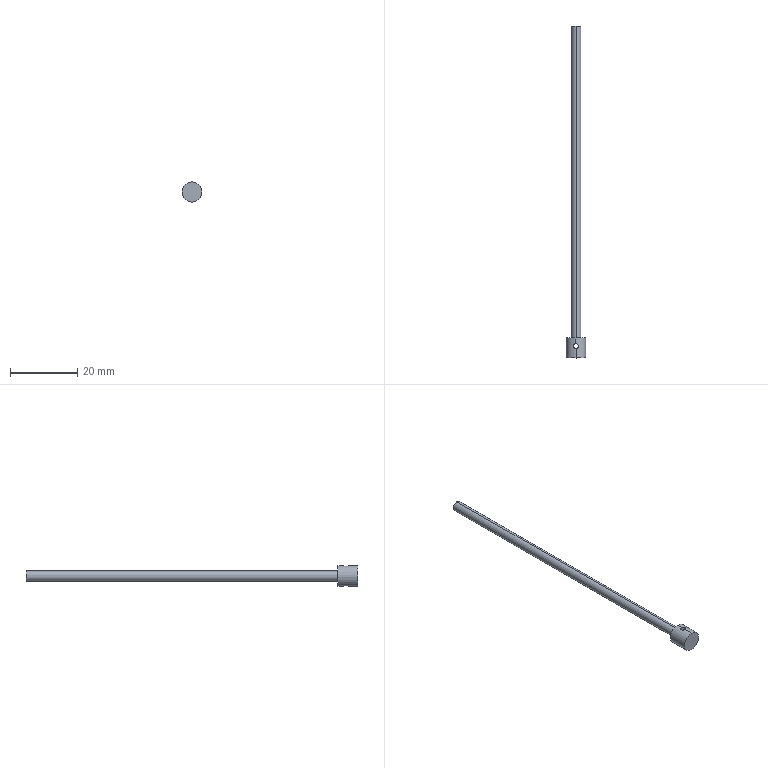Part | STEP file | magnetic tile detection pin | 1 solid | 9 faces | box 6 x 99 x 6 mm | volume 816.507 mm3 | cylinder 6 | plane 3 | commonest cylinder face diameters 1.5 x2 3 x2 6 x2
STEP:
#1=CARTESIAN_POINT('',(0.,0.,0.));
#2=DIRECTION('',(0.,0.,1.));
#3=DIRECTION('',(1.,0.,0.));
#4=AXIS2_PLACEMENT_3D('',#1,#2,#3);
#5=CARTESIAN_POINT('',(0.75,3.5,-2.905));
#6=VERTEX_POINT('',#5);
#7=CARTESIAN_POINT('',(0.,2.75,-3.));
#8=VERTEX_POINT('',#7);
#9=CARTESIAN_POINT('',(0.75,3.5,-2.905));
#10=CARTESIAN_POINT('',(0.75,3.402,-2.905));
#11=CARTESIAN_POINT('',(0.7304,3.303,-2.91));
#12=CARTESIAN_POINT('',(0.6548,3.121,-2.928));
#13=CARTESIAN_POINT('',(0.5996,3.039,-2.94));
#14=CARTESIAN_POINT('',(0.4606,2.9,-2.965));
#15=CARTESIAN_POINT('',(0.378,2.845,-2.977));
#16=CARTESIAN_POINT('',(0.1969,2.77,-2.995));
#17=CARTESIAN_POINT('',(0.0981,2.75,-3.));
#18=CARTESIAN_POINT('',(0.,2.75,-3.));
#19=B_SPLINE_CURVE_WITH_KNOTS('',3,(#9,#10,#11,#12,#13,#14,#15,#16,#17,#18),.UNSPECIFIED.,.F.,.F.,(4,2,2,2,4),(0.001177,0.001472,0.001766,0.00206,0.002354),.UNSPECIFIED.);
#20=CARTESIAN_POINT('',(0.,3.5,-5.));
#21=DIRECTION('',(0.,0.,1.));
#22=DIRECTION('',(1.,0.,0.));
#23=AXIS2_PLACEMENT_3D('',#20,#21,#22);
#24=CYLINDRICAL_SURFACE('',#23,0.75);
#25=CARTESIAN_POINT('',(6.283,2.095));
#26=CARTESIAN_POINT('',(6.259,2.095));
#27=CARTESIAN_POINT('',(6.212,2.095));
#28=CARTESIAN_POINT('',(6.14,2.093));
#29=CARTESIAN_POINT('',(6.069,2.091));
#30=CARTESIAN_POINT('',(5.997,2.088));
#31=CARTESIAN_POINT('',(5.925,2.084));
#32=CARTESIAN_POINT('',(5.854,2.079));
#33=CARTESIAN_POINT('',(5.782,2.073));
#34=CARTESIAN_POINT('',(5.711,2.067));
#35=CARTESIAN_POINT('',(5.64,2.061));
#36=CARTESIAN_POINT('',(5.569,2.054));
#37=CARTESIAN_POINT('',(5.497,2.047));
#38=CARTESIAN_POINT('',(5.426,2.04));
#39=CARTESIAN_POINT('',(5.355,2.034));
#40=CARTESIAN_POINT('',(5.284,2.027));
#41=CARTESIAN_POINT('',(5.213,2.022));
#42=CARTESIAN_POINT('',(5.141,2.016));
#43=CARTESIAN_POINT('',(5.07,2.011));
#44=CARTESIAN_POINT('',(4.999,2.007));
#45=CARTESIAN_POINT('',(4.927,2.004));
#46=CARTESIAN_POINT('',(4.855,2.002));
#47=CARTESIAN_POINT('',(4.784,2.));
#48=CARTESIAN_POINT('',(4.736,2.));
#49=CARTESIAN_POINT('',(4.712,2.));
#50=B_SPLINE_CURVE_WITH_KNOTS('',3,(#25,#26,#27,#28,#29,#30,#31,#32,#33,#34,#35,#36,#37,#38,#39,#40,#41,#42,#43,#44,#45,#46,#47,#48,#49),.UNSPECIFIED.,.F.,.F.,(4,1,1,1,1,1,1,1,1,1,1,1,1,1,1,1,1,1,1,1,1,1,4),(0.001177,0.001231,0.001284,0.001338,0.001391,0.001445,0.001498,0.001552,0.001605,0.001659,0.001712,0.001766,0.001819,0.001873,0.001926,0.00198,0.002033,0.002087,0.00214,0.002194,0.002247,0.002301,0.002354),.QUASI_UNIFORM_KNOTS.);
#51=(GEOMETRIC_REPRESENTATION_CONTEXT(2)PARAMETRIC_REPRESENTATION_CONTEXT()REPRESENTATION_CONTEXT('',''));
#52=DEFINITIONAL_REPRESENTATION('',(#50),#51);
#53=PCURVE('',#24,#52);
#54=CARTESIAN_POINT('',(0.,0.,0.));
#55=DIRECTION('',(0.,-1.,0.));
#56=DIRECTION('',(0.,0.,-1.));
#57=AXIS2_PLACEMENT_3D('',#54,#55,#56);
#58=CYLINDRICAL_SURFACE('',#57,3.);
#59=CARTESIAN_POINT('',(0.2527,-3.5));
#60=CARTESIAN_POINT('',(0.2527,-3.482));
#61=CARTESIAN_POINT('',(0.2522,-3.446));
#62=CARTESIAN_POINT('',(0.2502,-3.393));
#63=CARTESIAN_POINT('',(0.247,-3.34));
#64=CARTESIAN_POINT('',(0.2424,-3.288));
#65=CARTESIAN_POINT('',(0.2366,-3.237));
#66=CARTESIAN_POINT('',(0.2295,-3.187));
#67=CARTESIAN_POINT('',(0.2213,-3.14));
#68=CARTESIAN_POINT('',(0.2119,-3.094));
#69=CARTESIAN_POINT('',(0.2016,-3.05));
#70=CARTESIAN_POINT('',(0.1902,-3.008));
#71=CARTESIAN_POINT('',(0.1778,-2.969));
#72=CARTESIAN_POINT('',(0.1645,-2.933));
#73=CARTESIAN_POINT('',(0.1505,-2.899));
#74=CARTESIAN_POINT('',(0.1357,-2.869));
#75=CARTESIAN_POINT('',(0.1203,-2.841));
#76=CARTESIAN_POINT('',(0.1043,-2.817));
#77=CARTESIAN_POINT('',(0.08771,-2.797));
#78=CARTESIAN_POINT('',(0.07069,-2.78));
#79=CARTESIAN_POINT('',(0.0533,-2.767));
#80=CARTESIAN_POINT('',(0.03566,-2.757));
#81=CARTESIAN_POINT('',(0.01785,-2.751));
#82=CARTESIAN_POINT('',(0.005946,-2.75));
#83=CARTESIAN_POINT('',(0.,-2.75));
#84=B_SPLINE_CURVE_WITH_KNOTS('',3,(#59,#60,#61,#62,#63,#64,#65,#66,#67,#68,#69,#70,#71,#72,#73,#74,#75,#76,#77,#78,#79,#80,#81,#82,#83),.UNSPECIFIED.,.F.,.F.,(4,1,1,1,1,1,1,1,1,1,1,1,1,1,1,1,1,1,1,1,1,1,4),(0.001177,0.001231,0.001284,0.001338,0.001391,0.001445,0.001498,0.001552,0.001605,0.001659,0.001712,0.001766,0.001819,0.001873,0.001926,0.00198,0.002033,0.002087,0.00214,0.002194,0.002247,0.002301,0.002354),.QUASI_UNIFORM_KNOTS.);
#85=(GEOMETRIC_REPRESENTATION_CONTEXT(2)PARAMETRIC_REPRESENTATION_CONTEXT()REPRESENTATION_CONTEXT('',''));
#86=DEFINITIONAL_REPRESENTATION('',(#84),#85);
#87=PCURVE('',#58,#86);
#88=SURFACE_CURVE('',#19,(#53,#87),.PCURVE_S1.);
#89=EDGE_CURVE('',#6,#8,#88,.T.);
#90=ORIENTED_EDGE('',*,*,#89,.F.);
#91=CARTESIAN_POINT('',(0.75,3.5,2.905));
#92=VERTEX_POINT('',#91);
#93=CARTESIAN_POINT('',(0.75,3.5,-5.));
#94=DIRECTION('',(0.,0.,1.));
#95=VECTOR('',#94,1.);
#96=LINE('',#93,#95);
#97=CARTESIAN_POINT('',(6.283,0.));
#98=DIRECTION('',(0.,1.));
#99=VECTOR('',#98,1.);
#100=LINE('',#97,#99);
#101=(GEOMETRIC_REPRESENTATION_CONTEXT(2)PARAMETRIC_REPRESENTATION_CONTEXT()REPRESENTATION_CONTEXT('',''));
#102=DEFINITIONAL_REPRESENTATION('',(#100),#101);
#103=PCURVE('',#24,#102);
#104=CARTESIAN_POINT('',(0.,3.5,-5.));
#105=DIRECTION('',(0.,0.,1.));
#106=DIRECTION('',(1.,0.,0.));
#107=AXIS2_PLACEMENT_3D('',#104,#105,#106);
#108=CYLINDRICAL_SURFACE('',#107,0.75);
#109=CARTESIAN_POINT('',(0.,0.));
#110=DIRECTION('',(0.,1.));
#111=VECTOR('',#110,1.);
#112=LINE('',#109,#111);
#113=(GEOMETRIC_REPRESENTATION_CONTEXT(2)PARAMETRIC_REPRESENTATION_CONTEXT()REPRESENTATION_CONTEXT('',''));
#114=DEFINITIONAL_REPRESENTATION('',(#112),#113);
#115=PCURVE('',#108,#114);
#116=SURFACE_CURVE('',#96,(#103,#115),.PCURVE_S1.);
#117=EDGE_CURVE('',#6,#92,#116,.T.);
#118=ORIENTED_EDGE('',*,*,#117,.T.);
#119=CARTESIAN_POINT('',(0.,2.75,3.));
#120=VERTEX_POINT('',#119);
#121=CARTESIAN_POINT('',(0.,2.75,3.));
#122=CARTESIAN_POINT('',(0.1978,2.75,3.));
#123=CARTESIAN_POINT('',(0.3925,2.832,2.978));
#124=CARTESIAN_POINT('',(0.6678,3.107,2.928));
#125=CARTESIAN_POINT('',(0.75,3.301,2.905));
#126=CARTESIAN_POINT('',(0.75,3.5,2.905));
#127=B_SPLINE_CURVE_WITH_KNOTS('',3,(#121,#122,#123,#124,#125,#126),.UNSPECIFIED.,.F.,.F.,(4,2,4),(0.003531,0.004119,0.004708),.UNSPECIFIED.);
#128=CARTESIAN_POINT('',(4.712,8.));
#129=CARTESIAN_POINT('',(4.736,8.));
#130=CARTESIAN_POINT('',(4.784,8.));
#131=CARTESIAN_POINT('',(4.856,7.998));
#132=CARTESIAN_POINT('',(4.928,7.996));
#133=CARTESIAN_POINT('',(4.999,7.992));
#134=CARTESIAN_POINT('',(5.071,7.988));
#135=CARTESIAN_POINT('',(5.142,7.983));
#136=CARTESIAN_POINT('',(5.213,7.978));
#137=CARTESIAN_POINT('',(5.285,7.972));
#138=CARTESIAN_POINT('',(5.356,7.966));
#139=CARTESIAN_POINT('',(5.427,7.959));
#140=CARTESIAN_POINT('',(5.497,7.953));
#141=CARTESIAN_POINT('',(5.568,7.946));
#142=CARTESIAN_POINT('',(5.639,7.94));
#143=CARTESIAN_POINT('',(5.71,7.933));
#144=CARTESIAN_POINT('',(5.781,7.927));
#145=CARTESIAN_POINT('',(5.853,7.922));
#146=CARTESIAN_POINT('',(5.924,7.917));
#147=CARTESIAN_POINT('',(5.996,7.913));
#148=CARTESIAN_POINT('',(6.067,7.909));
#149=CARTESIAN_POINT('',(6.139,7.907));
#150=CARTESIAN_POINT('',(6.211,7.905));
#151=CARTESIAN_POINT('',(6.259,7.905));
#152=CARTESIAN_POINT('',(6.283,7.905));
#153=B_SPLINE_CURVE_WITH_KNOTS('',3,(#128,#129,#130,#131,#132,#133,#134,#135,#136,#137,#138,#139,#140,#141,#142,#143,#144,#145,#146,#147,#148,#149,#150,#151,#152),.UNSPECIFIED.,.F.,.F.,(4,1,1,1,1,1,1,1,1,1,1,1,1,1,1,1,1,1,1,1,1,1,4),(0.003531,0.003585,0.003638,0.003692,0.003745,0.003799,0.003852,0.003906,0.003959,0.004013,0.004066,0.004119,0.004173,0.004226,0.00428,0.004333,0.004387,0.00444,0.004494,0.004547,0.004601,0.004654,0.004708),.QUASI_UNIFORM_KNOTS.);
#154=(GEOMETRIC_REPRESENTATION_CONTEXT(2)PARAMETRIC_REPRESENTATION_CONTEXT()REPRESENTATION_CONTEXT('',''));
#155=DEFINITIONAL_REPRESENTATION('',(#153),#154);
#156=PCURVE('',#24,#155);
#157=CARTESIAN_POINT('',(3.142,-2.75));
#158=CARTESIAN_POINT('',(3.136,-2.75));
#159=CARTESIAN_POINT('',(3.124,-2.751));
#160=CARTESIAN_POINT('',(3.106,-2.757));
#161=CARTESIAN_POINT('',(3.088,-2.767));
#162=CARTESIAN_POINT('',(3.071,-2.781));
#163=CARTESIAN_POINT('',(3.054,-2.798));
#164=CARTESIAN_POINT('',(3.037,-2.818));
#165=CARTESIAN_POINT('',(3.021,-2.842));
#166=CARTESIAN_POINT('',(3.006,-2.869));
#167=CARTESIAN_POINT('',(2.991,-2.9));
#168=CARTESIAN_POINT('',(2.977,-2.933));
#169=CARTESIAN_POINT('',(2.964,-2.969));
#170=CARTESIAN_POINT('',(2.952,-3.008));
#171=CARTESIAN_POINT('',(2.94,-3.049));
#172=CARTESIAN_POINT('',(2.93,-3.093));
#173=CARTESIAN_POINT('',(2.921,-3.139));
#174=CARTESIAN_POINT('',(2.912,-3.187));
#175=CARTESIAN_POINT('',(2.905,-3.236));
#176=CARTESIAN_POINT('',(2.899,-3.287));
#177=CARTESIAN_POINT('',(2.895,-3.339));
#178=CARTESIAN_POINT('',(2.891,-3.392));
#179=CARTESIAN_POINT('',(2.889,-3.446));
#180=CARTESIAN_POINT('',(2.889,-3.482));
#181=CARTESIAN_POINT('',(2.889,-3.5));
#182=B_SPLINE_CURVE_WITH_KNOTS('',3,(#157,#158,#159,#160,#161,#162,#163,#164,#165,#166,#167,#168,#169,#170,#171,#172,#173,#174,#175,#176,#177,#178,#179,#180,#181),.UNSPECIFIED.,.F.,.F.,(4,1,1,1,1,1,1,1,1,1,1,1,1,1,1,1,1,1,1,1,1,1,4),(0.003531,0.003585,0.003638,0.003692,0.003745,0.003799,0.003852,0.003906,0.003959,0.004013,0.004066,0.004119,0.004173,0.004226,0.00428,0.004333,0.004387,0.00444,0.004494,0.004547,0.004601,0.004654,0.004708),.QUASI_UNIFORM_KNOTS.);
#183=(GEOMETRIC_REPRESENTATION_CONTEXT(2)PARAMETRIC_REPRESENTATION_CONTEXT()REPRESENTATION_CONTEXT('',''));
#184=DEFINITIONAL_REPRESENTATION('',(#182),#183);
#185=PCURVE('',#58,#184);
#186=SURFACE_CURVE('',#127,(#156,#185),.PCURVE_S1.);
#187=EDGE_CURVE('',#120,#92,#186,.T.);
#188=ORIENTED_EDGE('',*,*,#187,.F.);
#189=CARTESIAN_POINT('',(-0.75,3.5,2.905));
#190=VERTEX_POINT('',#189);
#191=CARTESIAN_POINT('',(-0.75,3.5,2.905));
#192=CARTESIAN_POINT('',(-0.75,3.402,2.905));
#193=CARTESIAN_POINT('',(-0.7302,3.303,2.91));
#194=CARTESIAN_POINT('',(-0.6552,3.122,2.928));
#195=CARTESIAN_POINT('',(-0.5996,3.039,2.94));
#196=CARTESIAN_POINT('',(-0.3922,2.831,2.978));
#197=CARTESIAN_POINT('',(-0.1979,2.75,3.));
#198=CARTESIAN_POINT('',(0.,2.75,3.));
#199=B_SPLINE_CURVE_WITH_KNOTS('',3,(#191,#192,#193,#194,#195,#196,#197,#198),.UNSPECIFIED.,.F.,.F.,(4,2,2,4),(0.002354,0.002648,0.002943,0.003531),.UNSPECIFIED.);
#200=CARTESIAN_POINT('',(3.142,7.905));
#201=CARTESIAN_POINT('',(3.165,7.905));
#202=CARTESIAN_POINT('',(3.213,7.905));
#203=CARTESIAN_POINT('',(3.285,7.907));
#204=CARTESIAN_POINT('',(3.356,7.909));
#205=CARTESIAN_POINT('',(3.428,7.912));
#206=CARTESIAN_POINT('',(3.499,7.916));
#207=CARTESIAN_POINT('',(3.571,7.921));
#208=CARTESIAN_POINT('',(3.642,7.927));
#209=CARTESIAN_POINT('',(3.713,7.933));
#210=CARTESIAN_POINT('',(3.784,7.939));
#211=CARTESIAN_POINT('',(3.855,7.946));
#212=CARTESIAN_POINT('',(3.927,7.953));
#213=CARTESIAN_POINT('',(3.998,7.959));
#214=CARTESIAN_POINT('',(4.069,7.966));
#215=CARTESIAN_POINT('',(4.14,7.972));
#216=CARTESIAN_POINT('',(4.211,7.978));
#217=CARTESIAN_POINT('',(4.283,7.983));
#218=CARTESIAN_POINT('',(4.354,7.988));
#219=CARTESIAN_POINT('',(4.426,7.992));
#220=CARTESIAN_POINT('',(4.497,7.996));
#221=CARTESIAN_POINT('',(4.569,7.998));
#222=CARTESIAN_POINT('',(4.641,8.));
#223=CARTESIAN_POINT('',(4.688,8.));
#224=CARTESIAN_POINT('',(4.712,8.));
#225=B_SPLINE_CURVE_WITH_KNOTS('',3,(#200,#201,#202,#203,#204,#205,#206,#207,#208,#209,#210,#211,#212,#213,#214,#215,#216,#217,#218,#219,#220,#221,#222,#223,#224),.UNSPECIFIED.,.F.,.F.,(4,1,1,1,1,1,1,1,1,1,1,1,1,1,1,1,1,1,1,1,1,1,4),(0.002354,0.002408,0.002461,0.002515,0.002568,0.002622,0.002675,0.002729,0.002782,0.002836,0.002889,0.002943,0.002996,0.00305,0.003103,0.003157,0.00321,0.003264,0.003317,0.003371,0.003424,0.003478,0.003531),.QUASI_UNIFORM_KNOTS.);
#226=(GEOMETRIC_REPRESENTATION_CONTEXT(2)PARAMETRIC_REPRESENTATION_CONTEXT()REPRESENTATION_CONTEXT('',''));
#227=DEFINITIONAL_REPRESENTATION('',(#225),#226);
#228=PCURVE('',#24,#227);
#229=CARTESIAN_POINT('',(0.,0.,0.));
#230=DIRECTION('',(0.,-1.,0.));
#231=DIRECTION('',(0.,0.,-1.));
#232=AXIS2_PLACEMENT_3D('',#229,#230,#231);
#233=CYLINDRICAL_SURFACE('',#232,3.);
#234=CARTESIAN_POINT('',(3.394,-3.5));
#235=CARTESIAN_POINT('',(3.394,-3.482));
#236=CARTESIAN_POINT('',(3.394,-3.446));
#237=CARTESIAN_POINT('',(3.392,-3.393));
#238=CARTESIAN_POINT('',(3.389,-3.34));
#239=CARTESIAN_POINT('',(3.384,-3.288));
#240=CARTESIAN_POINT('',(3.378,-3.237));
#241=CARTESIAN_POINT('',(3.371,-3.188));
#242=CARTESIAN_POINT('',(3.363,-3.14));
#243=CARTESIAN_POINT('',(3.354,-3.094));
#244=CARTESIAN_POINT('',(3.343,-3.05));
#245=CARTESIAN_POINT('',(3.332,-3.009));
#246=CARTESIAN_POINT('',(3.32,-2.969));
#247=CARTESIAN_POINT('',(3.306,-2.933));
#248=CARTESIAN_POINT('',(3.292,-2.9));
#249=CARTESIAN_POINT('',(3.277,-2.869));
#250=CARTESIAN_POINT('',(3.262,-2.842));
#251=CARTESIAN_POINT('',(3.246,-2.818));
#252=CARTESIAN_POINT('',(3.229,-2.798));
#253=CARTESIAN_POINT('',(3.212,-2.781));
#254=CARTESIAN_POINT('',(3.195,-2.767));
#255=CARTESIAN_POINT('',(3.177,-2.757));
#256=CARTESIAN_POINT('',(3.16,-2.751));
#257=CARTESIAN_POINT('',(3.148,-2.75));
#258=CARTESIAN_POINT('',(3.142,-2.75));
#259=B_SPLINE_CURVE_WITH_KNOTS('',3,(#234,#235,#236,#237,#238,#239,#240,#241,#242,#243,#244,#245,#246,#247,#248,#249,#250,#251,#252,#253,#254,#255,#256,#257,#258),.UNSPECIFIED.,.F.,.F.,(4,1,1,1,1,1,1,1,1,1,1,1,1,1,1,1,1,1,1,1,1,1,4),(0.002354,0.002408,0.002461,0.002515,0.002568,0.002622,0.002675,0.002729,0.002782,0.002836,0.002889,0.002943,0.002996,0.00305,0.003103,0.003157,0.00321,0.003264,0.003317,0.003371,0.003424,0.003478,0.003531),.QUASI_UNIFORM_KNOTS.);
#260=(GEOMETRIC_REPRESENTATION_CONTEXT(2)PARAMETRIC_REPRESENTATION_CONTEXT()REPRESENTATION_CONTEXT('',''));
#261=DEFINITIONAL_REPRESENTATION('',(#259),#260);
#262=PCURVE('',#233,#261);
#263=SURFACE_CURVE('',#199,(#228,#262),.PCURVE_S1.);
#264=EDGE_CURVE('',#190,#120,#263,.T.);
#265=ORIENTED_EDGE('',*,*,#264,.F.);
#266=CARTESIAN_POINT('',(-0.75,3.5,-2.905));
#267=VERTEX_POINT('',#266);
#268=CARTESIAN_POINT('',(-0.75,3.5,-5.));
#269=DIRECTION('',(0.,0.,1.));
#270=VECTOR('',#269,1.);
#271=LINE('',#268,#270);
#272=CARTESIAN_POINT('',(3.142,0.));
#273=DIRECTION('',(0.,1.));
#274=VECTOR('',#273,1.);
#275=LINE('',#272,#274);
#276=(GEOMETRIC_REPRESENTATION_CONTEXT(2)PARAMETRIC_REPRESENTATION_CONTEXT()REPRESENTATION_CONTEXT('',''));
#277=DEFINITIONAL_REPRESENTATION('',(#275),#276);
#278=PCURVE('',#24,#277);
#279=CARTESIAN_POINT('',(3.142,0.));
#280=DIRECTION('',(0.,1.));
#281=VECTOR('',#280,1.);
#282=LINE('',#279,#281);
#283=(GEOMETRIC_REPRESENTATION_CONTEXT(2)PARAMETRIC_REPRESENTATION_CONTEXT()REPRESENTATION_CONTEXT('',''));
#284=DEFINITIONAL_REPRESENTATION('',(#282),#283);
#285=PCURVE('',#108,#284);
#286=SURFACE_CURVE('',#271,(#278,#285),.PCURVE_S1.);
#287=EDGE_CURVE('',#267,#190,#286,.T.);
#288=ORIENTED_EDGE('',*,*,#287,.F.);
#289=CARTESIAN_POINT('',(0.,2.75,-3.));
#290=CARTESIAN_POINT('',(-0.09812,2.75,-3.));
#291=CARTESIAN_POINT('',(-0.1972,2.77,-2.995));
#292=CARTESIAN_POINT('',(-0.3779,2.845,-2.977));
#293=CARTESIAN_POINT('',(-0.461,2.9,-2.965));
#294=CARTESIAN_POINT('',(-0.6686,3.108,-2.928));
#295=CARTESIAN_POINT('',(-0.75,3.302,-2.905));
#296=CARTESIAN_POINT('',(-0.75,3.5,-2.905));
#297=B_SPLINE_CURVE_WITH_KNOTS('',3,(#289,#290,#291,#292,#293,#294,#295,#296),.UNSPECIFIED.,.F.,.F.,(4,2,2,4),(0.002354,0.002648,0.002943,0.003531),.UNSPECIFIED.);
#298=CARTESIAN_POINT('',(4.712,2.));
#299=CARTESIAN_POINT('',(4.689,2.));
#300=CARTESIAN_POINT('',(4.641,2.));
#301=CARTESIAN_POINT('',(4.569,2.002));
#302=CARTESIAN_POINT('',(4.498,2.004));
#303=CARTESIAN_POINT('',(4.426,2.007));
#304=CARTESIAN_POINT('',(4.354,2.011));
#305=CARTESIAN_POINT('',(4.283,2.016));
#306=CARTESIAN_POINT('',(4.212,2.022));
#307=CARTESIAN_POINT('',(4.141,2.028));
#308=CARTESIAN_POINT('',(4.07,2.034));
#309=CARTESIAN_POINT('',(3.998,2.04));
#310=CARTESIAN_POINT('',(3.927,2.047));
#311=CARTESIAN_POINT('',(3.856,2.054));
#312=CARTESIAN_POINT('',(3.785,2.061));
#313=CARTESIAN_POINT('',(3.714,2.067));
#314=CARTESIAN_POINT('',(3.643,2.073));
#315=CARTESIAN_POINT('',(3.571,2.078));
#316=CARTESIAN_POINT('',(3.5,2.083));
#317=CARTESIAN_POINT('',(3.428,2.087));
#318=CARTESIAN_POINT('',(3.357,2.091));
#319=CARTESIAN_POINT('',(3.285,2.093));
#320=CARTESIAN_POINT('',(3.213,2.095));
#321=CARTESIAN_POINT('',(3.166,2.095));
#322=CARTESIAN_POINT('',(3.142,2.095));
#323=B_SPLINE_CURVE_WITH_KNOTS('',3,(#298,#299,#300,#301,#302,#303,#304,#305,#306,#307,#308,#309,#310,#311,#312,#313,#314,#315,#316,#317,#318,#319,#320,#321,#322),.UNSPECIFIED.,.F.,.F.,(4,1,1,1,1,1,1,1,1,1,1,1,1,1,1,1,1,1,1,1,1,1,4),(0.002354,0.002408,0.002461,0.002515,0.002568,0.002622,0.002675,0.002729,0.002782,0.002836,0.002889,0.002943,0.002996,0.00305,0.003103,0.003157,0.00321,0.003264,0.003317,0.003371,0.003424,0.003478,0.003531),.QUASI_UNIFORM_KNOTS.);
#324=(GEOMETRIC_REPRESENTATION_CONTEXT(2)PARAMETRIC_REPRESENTATION_CONTEXT()REPRESENTATION_CONTEXT('',''));
#325=DEFINITIONAL_REPRESENTATION('',(#323),#324);
#326=PCURVE('',#24,#325);
#327=CARTESIAN_POINT('',(6.283,-2.75));
#328=CARTESIAN_POINT('',(6.277,-2.75));
#329=CARTESIAN_POINT('',(6.265,-2.751));
#330=CARTESIAN_POINT('',(6.247,-2.757));
#331=CARTESIAN_POINT('',(6.23,-2.767));
#332=CARTESIAN_POINT('',(6.212,-2.78));
#333=CARTESIAN_POINT('',(6.195,-2.797));
#334=CARTESIAN_POINT('',(6.179,-2.817));
#335=CARTESIAN_POINT('',(6.163,-2.841));
#336=CARTESIAN_POINT('',(6.147,-2.869));
#337=CARTESIAN_POINT('',(6.133,-2.899));
#338=CARTESIAN_POINT('',(6.119,-2.933));
#339=CARTESIAN_POINT('',(6.105,-2.969));
#340=CARTESIAN_POINT('',(6.093,-3.008));
#341=CARTESIAN_POINT('',(6.082,-3.05));
#342=CARTESIAN_POINT('',(6.071,-3.094));
#343=CARTESIAN_POINT('',(6.062,-3.14));
#344=CARTESIAN_POINT('',(6.054,-3.188));
#345=CARTESIAN_POINT('',(6.047,-3.237));
#346=CARTESIAN_POINT('',(6.041,-3.288));
#347=CARTESIAN_POINT('',(6.036,-3.34));
#348=CARTESIAN_POINT('',(6.033,-3.393));
#349=CARTESIAN_POINT('',(6.031,-3.446));
#350=CARTESIAN_POINT('',(6.031,-3.482));
#351=CARTESIAN_POINT('',(6.031,-3.5));
#352=B_SPLINE_CURVE_WITH_KNOTS('',3,(#327,#328,#329,#330,#331,#332,#333,#334,#335,#336,#337,#338,#339,#340,#341,#342,#343,#344,#345,#346,#347,#348,#349,#350,#351),.UNSPECIFIED.,.F.,.F.,(4,1,1,1,1,1,1,1,1,1,1,1,1,1,1,1,1,1,1,1,1,1,4),(0.002354,0.002408,0.002461,0.002515,0.002568,0.002622,0.002675,0.002729,0.002782,0.002836,0.002889,0.002943,0.002996,0.00305,0.003103,0.003157,0.00321,0.003264,0.003317,0.003371,0.003424,0.003478,0.003531),.QUASI_UNIFORM_KNOTS.);
#353=(GEOMETRIC_REPRESENTATION_CONTEXT(2)PARAMETRIC_REPRESENTATION_CONTEXT()REPRESENTATION_CONTEXT('',''));
#354=DEFINITIONAL_REPRESENTATION('',(#352),#353);
#355=PCURVE('',#233,#354);
#356=SURFACE_CURVE('',#297,(#326,#355),.PCURVE_S1.);
#357=EDGE_CURVE('',#8,#267,#356,.T.);
#358=ORIENTED_EDGE('',*,*,#357,.F.);
#359=EDGE_LOOP('',(#90,#118,#188,#265,#288,#358));
#360=FACE_BOUND('',#359,.F.);
#361=ADVANCED_FACE('',(#360),#24,.F.);
#362=CARTESIAN_POINT('',(0.,99.,-1.5));
#363=VERTEX_POINT('',#362);
#364=CARTESIAN_POINT('',(0.,99.,1.5));
#365=VERTEX_POINT('',#364);
#366=CARTESIAN_POINT('',(0.,99.,0.));
#367=DIRECTION('',(0.,-1.,0.));
#368=DIRECTION('',(0.,0.,-1.));
#369=AXIS2_PLACEMENT_3D('',#366,#367,#368);
#370=CIRCLE('',#369,1.5);
#371=CARTESIAN_POINT('',(0.,0.,0.));
#372=DIRECTION('',(0.,-1.,0.));
#373=DIRECTION('',(0.,0.,-1.));
#374=AXIS2_PLACEMENT_3D('',#371,#372,#373);
#375=CYLINDRICAL_SURFACE('',#374,1.5);
#376=CARTESIAN_POINT('',(0.,-99.));
#377=DIRECTION('',(1.,0.));
#378=VECTOR('',#377,1.);
#379=LINE('',#376,#378);
#380=(GEOMETRIC_REPRESENTATION_CONTEXT(2)PARAMETRIC_REPRESENTATION_CONTEXT()REPRESENTATION_CONTEXT('',''));
#381=DEFINITIONAL_REPRESENTATION('',(#379),#380);
#382=PCURVE('',#375,#381);
#383=CARTESIAN_POINT('',(1.5,99.,0.));
#384=DIRECTION('',(0.,1.,0.));
#385=DIRECTION('',(0.,0.,1.));
#386=AXIS2_PLACEMENT_3D('',#383,#384,#385);
#387=PLANE('',#386);
#388=CARTESIAN_POINT('',(-1.5,-1.5));
#389=CARTESIAN_POINT('',(-1.5,1.098));
#390=CARTESIAN_POINT('',(0.75,-0.201));
#391=CARTESIAN_POINT('',(3.,-1.5));
#392=CARTESIAN_POINT('',(0.75,-2.799));
#393=CARTESIAN_POINT('',(-1.5,-4.098));
#394=CARTESIAN_POINT('',(-1.5,-1.5));
#395=(BOUNDED_CURVE()B_SPLINE_CURVE(2,(#388,#389,#390,#391,#392,#393,#394),.UNSPECIFIED.,.T.,.F.)B_SPLINE_CURVE_WITH_KNOTS((1,2,2,2,2,1),(-2.094,0.,2.094,4.189,6.283,8.378),.UNSPECIFIED.)CURVE()GEOMETRIC_REPRESENTATION_ITEM()RATIONAL_B_SPLINE_CURVE((1.,0.5,1.,0.5,1.,0.5,1.))REPRESENTATION_ITEM(''));
#396=(GEOMETRIC_REPRESENTATION_CONTEXT(2)PARAMETRIC_REPRESENTATION_CONTEXT()REPRESENTATION_CONTEXT('',''));
#397=DEFINITIONAL_REPRESENTATION('',(#395),#396);
#398=PCURVE('',#387,#397);
#399=SURFACE_CURVE('',#370,(#382,#398),.PCURVE_S1.);
#400=EDGE_CURVE('',#363,#365,#399,.T.);
#401=ORIENTED_EDGE('',*,*,#400,.T.);
#402=CARTESIAN_POINT('',(0.,6.,1.5));
#403=VERTEX_POINT('',#402);
#404=CARTESIAN_POINT('',(0.,0.,1.5));
#405=DIRECTION('',(0.,-1.,0.));
#406=VECTOR('',#405,1.);
#407=LINE('',#404,#406);
#408=CARTESIAN_POINT('',(3.142,0.));
#409=DIRECTION('',(0.,1.));
#410=VECTOR('',#409,1.);
#411=LINE('',#408,#410);
#412=(GEOMETRIC_REPRESENTATION_CONTEXT(2)PARAMETRIC_REPRESENTATION_CONTEXT()REPRESENTATION_CONTEXT('',''));
#413=DEFINITIONAL_REPRESENTATION('',(#411),#412);
#414=PCURVE('',#375,#413);
#415=CARTESIAN_POINT('',(0.,0.,0.));
#416=DIRECTION('',(0.,-1.,0.));
#417=DIRECTION('',(0.,0.,-1.));
#418=AXIS2_PLACEMENT_3D('',#415,#416,#417);
#419=CYLINDRICAL_SURFACE('',#418,1.5);
#420=CARTESIAN_POINT('',(3.142,0.));
#421=DIRECTION('',(0.,1.));
#422=VECTOR('',#421,1.);
#423=LINE('',#420,#422);
#424=(GEOMETRIC_REPRESENTATION_CONTEXT(2)PARAMETRIC_REPRESENTATION_CONTEXT()REPRESENTATION_CONTEXT('',''));
#425=DEFINITIONAL_REPRESENTATION('',(#423),#424);
#426=PCURVE('',#419,#425);
#427=SURFACE_CURVE('',#407,(#414,#426),.PCURVE_S1.);
#428=EDGE_CURVE('',#365,#403,#427,.T.);
#429=ORIENTED_EDGE('',*,*,#428,.T.);
#430=CARTESIAN_POINT('',(0.,6.,-1.5));
#431=VERTEX_POINT('',#430);
#432=CARTESIAN_POINT('',(0.,6.,0.));
#433=DIRECTION('',(0.,-1.,0.));
#434=DIRECTION('',(0.,0.,-1.));
#435=AXIS2_PLACEMENT_3D('',#432,#433,#434);
#436=CIRCLE('',#435,1.5);
#437=CARTESIAN_POINT('',(0.,-6.));
#438=DIRECTION('',(1.,0.));
#439=VECTOR('',#438,1.);
#440=LINE('',#437,#439);
#441=(GEOMETRIC_REPRESENTATION_CONTEXT(2)PARAMETRIC_REPRESENTATION_CONTEXT()REPRESENTATION_CONTEXT('',''));
#442=DEFINITIONAL_REPRESENTATION('',(#440),#441);
#443=PCURVE('',#375,#442);
#444=CARTESIAN_POINT('',(3.,6.,0.));
#445=DIRECTION('',(0.,1.,0.));
#446=DIRECTION('',(0.,0.,1.));
#447=AXIS2_PLACEMENT_3D('',#444,#445,#446);
#448=PLANE('',#447);
#449=CARTESIAN_POINT('',(-1.5,-3.));
#450=CARTESIAN_POINT('',(-1.5,-0.4019));
#451=CARTESIAN_POINT('',(0.75,-1.701));
#452=CARTESIAN_POINT('',(3.,-3.));
#453=CARTESIAN_POINT('',(0.75,-4.299));
#454=CARTESIAN_POINT('',(-1.5,-5.598));
#455=CARTESIAN_POINT('',(-1.5,-3.));
#456=(BOUNDED_CURVE()B_SPLINE_CURVE(2,(#449,#450,#451,#452,#453,#454,#455),.UNSPECIFIED.,.T.,.F.)B_SPLINE_CURVE_WITH_KNOTS((1,2,2,2,2,1),(-2.094,0.,2.094,4.189,6.283,8.378),.UNSPECIFIED.)CURVE()GEOMETRIC_REPRESENTATION_ITEM()RATIONAL_B_SPLINE_CURVE((1.,0.5,1.,0.5,1.,0.5,1.))REPRESENTATION_ITEM(''));
#457=(GEOMETRIC_REPRESENTATION_CONTEXT(2)PARAMETRIC_REPRESENTATION_CONTEXT()REPRESENTATION_CONTEXT('',''));
#458=DEFINITIONAL_REPRESENTATION('',(#456),#457);
#459=PCURVE('',#448,#458);
#460=SURFACE_CURVE('',#436,(#443,#459),.PCURVE_S1.);
#461=EDGE_CURVE('',#431,#403,#460,.T.);
#462=ORIENTED_EDGE('',*,*,#461,.F.);
#463=CARTESIAN_POINT('',(0.,0.,-1.5));
#464=DIRECTION('',(0.,-1.,0.));
#465=VECTOR('',#464,1.);
#466=LINE('',#463,#465);
#467=CARTESIAN_POINT('',(0.,0.));
#468=DIRECTION('',(0.,1.));
#469=VECTOR('',#468,1.);
#470=LINE('',#467,#469);
#471=(GEOMETRIC_REPRESENTATION_CONTEXT(2)PARAMETRIC_REPRESENTATION_CONTEXT()REPRESENTATION_CONTEXT('',''));
#472=DEFINITIONAL_REPRESENTATION('',(#470),#471);
#473=PCURVE('',#375,#472);
#474=CARTESIAN_POINT('',(6.283,0.));
#475=DIRECTION('',(0.,1.));
#476=VECTOR('',#475,1.);
#477=LINE('',#474,#476);
#478=(GEOMETRIC_REPRESENTATION_CONTEXT(2)PARAMETRIC_REPRESENTATION_CONTEXT()REPRESENTATION_CONTEXT('',''));
#479=DEFINITIONAL_REPRESENTATION('',(#477),#478);
#480=PCURVE('',#419,#479);
#481=SURFACE_CURVE('',#466,(#473,#480),.PCURVE_S1.);
#482=EDGE_CURVE('',#363,#431,#481,.T.);
#483=ORIENTED_EDGE('',*,*,#482,.F.);
#484=EDGE_LOOP('',(#401,#429,#462,#483));
#485=FACE_BOUND('',#484,.T.);
#486=ADVANCED_FACE('',(#485),#375,.T.);
#487=CARTESIAN_POINT('',(0.,6.,-3.));
#488=VERTEX_POINT('',#487);
#489=CARTESIAN_POINT('',(0.,6.,3.));
#490=VERTEX_POINT('',#489);
#491=CARTESIAN_POINT('',(0.,6.,0.));
#492=DIRECTION('',(0.,-1.,0.));
#493=DIRECTION('',(0.,0.,-1.));
#494=AXIS2_PLACEMENT_3D('',#491,#492,#493);
#495=CIRCLE('',#494,3.);
#496=CARTESIAN_POINT('',(0.,-6.));
#497=DIRECTION('',(1.,0.));
#498=VECTOR('',#497,1.);
#499=LINE('',#496,#498);
#500=(GEOMETRIC_REPRESENTATION_CONTEXT(2)PARAMETRIC_REPRESENTATION_CONTEXT()REPRESENTATION_CONTEXT('',''));
#501=DEFINITIONAL_REPRESENTATION('',(#499),#500);
#502=PCURVE('',#58,#501);
#503=CARTESIAN_POINT('',(-3.,-3.));
#504=CARTESIAN_POINT('',(-3.,2.196));
#505=CARTESIAN_POINT('',(1.5,-0.4019));
#506=CARTESIAN_POINT('',(6.,-3.));
#507=CARTESIAN_POINT('',(1.5,-5.598));
#508=CARTESIAN_POINT('',(-3.,-8.196));
#509=CARTESIAN_POINT('',(-3.,-3.));
#510=(BOUNDED_CURVE()B_SPLINE_CURVE(2,(#503,#504,#505,#506,#507,#508,#509),.UNSPECIFIED.,.T.,.F.)B_SPLINE_CURVE_WITH_KNOTS((1,2,2,2,2,1),(-2.094,0.,2.094,4.189,6.283,8.378),.UNSPECIFIED.)CURVE()GEOMETRIC_REPRESENTATION_ITEM()RATIONAL_B_SPLINE_CURVE((1.,0.5,1.,0.5,1.,0.5,1.))REPRESENTATION_ITEM(''));
#511=(GEOMETRIC_REPRESENTATION_CONTEXT(2)PARAMETRIC_REPRESENTATION_CONTEXT()REPRESENTATION_CONTEXT('',''));
#512=DEFINITIONAL_REPRESENTATION('',(#510),#511);
#513=PCURVE('',#448,#512);
#514=SURFACE_CURVE('',#495,(#502,#513),.PCURVE_S1.);
#515=EDGE_CURVE('',#488,#490,#514,.T.);
#516=ORIENTED_EDGE('',*,*,#515,.T.);
#517=CARTESIAN_POINT('',(0.,4.25,3.));
#518=VERTEX_POINT('',#517);
#519=CARTESIAN_POINT('',(0.,0.,3.));
#520=DIRECTION('',(0.,-1.,0.));
#521=VECTOR('',#520,1.);
#522=LINE('',#519,#521);
#523=CARTESIAN_POINT('',(3.142,0.));
#524=DIRECTION('',(0.,1.));
#525=VECTOR('',#524,1.);
#526=LINE('',#523,#525);
#527=(GEOMETRIC_REPRESENTATION_CONTEXT(2)PARAMETRIC_REPRESENTATION_CONTEXT()REPRESENTATION_CONTEXT('',''));
#528=DEFINITIONAL_REPRESENTATION('',(#526),#527);
#529=PCURVE('',#58,#528);
#530=CARTESIAN_POINT('',(3.142,0.));
#531=DIRECTION('',(0.,1.));
#532=VECTOR('',#531,1.);
#533=LINE('',#530,#532);
#534=(GEOMETRIC_REPRESENTATION_CONTEXT(2)PARAMETRIC_REPRESENTATION_CONTEXT()REPRESENTATION_CONTEXT('',''));
#535=DEFINITIONAL_REPRESENTATION('',(#533),#534);
#536=PCURVE('',#233,#535);
#537=SURFACE_CURVE('',#522,(#529,#536),.PCURVE_S1.);
#538=EDGE_CURVE('',#490,#518,#537,.T.);
#539=ORIENTED_EDGE('',*,*,#538,.T.);
#540=CARTESIAN_POINT('',(0.75,3.5,2.905));
#541=CARTESIAN_POINT('',(0.75,3.6,2.905));
#542=CARTESIAN_POINT('',(0.7302,3.697,2.91));
#543=CARTESIAN_POINT('',(0.6548,3.879,2.928));
#544=CARTESIAN_POINT('',(0.599,3.962,2.94));
#545=CARTESIAN_POINT('',(0.4612,4.099,2.965));
#546=CARTESIAN_POINT('',(0.3778,4.155,2.978));
#547=CARTESIAN_POINT('',(0.1973,4.23,2.995));
#548=CARTESIAN_POINT('',(0.09831,4.25,3.));
#549=CARTESIAN_POINT('',(0.,4.25,3.));
#550=B_SPLINE_CURVE_WITH_KNOTS('',3,(#540,#541,#542,#543,#544,#545,#546,#547,#548,#549),.UNSPECIFIED.,.F.,.F.,(4,2,2,2,4),(0.,0.0002944,0.0005887,0.0008831,0.001177),.UNSPECIFIED.);
#551=CARTESIAN_POINT('',(2.889,-3.5));
#552=CARTESIAN_POINT('',(2.889,-3.518));
#553=CARTESIAN_POINT('',(2.889,-3.554));
#554=CARTESIAN_POINT('',(2.891,-3.608));
#555=CARTESIAN_POINT('',(2.895,-3.661));
#556=CARTESIAN_POINT('',(2.899,-3.712));
#557=CARTESIAN_POINT('',(2.905,-3.763));
#558=CARTESIAN_POINT('',(2.912,-3.813));
#559=CARTESIAN_POINT('',(2.92,-3.861));
#560=CARTESIAN_POINT('',(2.93,-3.907));
#561=CARTESIAN_POINT('',(2.94,-3.951));
#562=CARTESIAN_POINT('',(2.952,-3.992));
#563=CARTESIAN_POINT('',(2.964,-4.031));
#564=CARTESIAN_POINT('',(2.977,-4.067));
#565=CARTESIAN_POINT('',(2.991,-4.101));
#566=CARTESIAN_POINT('',(3.006,-4.131));
#567=CARTESIAN_POINT('',(3.021,-4.159));
#568=CARTESIAN_POINT('',(3.037,-4.183));
#569=CARTESIAN_POINT('',(3.054,-4.203));
#570=CARTESIAN_POINT('',(3.071,-4.22));
#571=CARTESIAN_POINT('',(3.088,-4.233));
#572=CARTESIAN_POINT('',(3.106,-4.243));
#573=CARTESIAN_POINT('',(3.124,-4.249));
#574=CARTESIAN_POINT('',(3.136,-4.25));
#575=CARTESIAN_POINT('',(3.142,-4.25));
#576=B_SPLINE_CURVE_WITH_KNOTS('',3,(#551,#552,#553,#554,#555,#556,#557,#558,#559,#560,#561,#562,#563,#564,#565,#566,#567,#568,#569,#570,#571,#572,#573,#574,#575),.UNSPECIFIED.,.F.,.F.,(4,1,1,1,1,1,1,1,1,1,1,1,1,1,1,1,1,1,1,1,1,1,4),(0.,0.00005352,0.000107,0.0001606,0.0002141,0.0002676,0.0003211,0.0003746,0.0004281,0.0004817,0.0005352,0.0005887,0.0006422,0.0006957,0.0007493,0.0008028,0.0008563,0.0009098,0.0009633,0.001017,0.00107,0.001124,0.001177),.QUASI_UNIFORM_KNOTS.);
#577=(GEOMETRIC_REPRESENTATION_CONTEXT(2)PARAMETRIC_REPRESENTATION_CONTEXT()REPRESENTATION_CONTEXT('',''));
#578=DEFINITIONAL_REPRESENTATION('',(#576),#577);
#579=PCURVE('',#58,#578);
#580=CARTESIAN_POINT('',(0.,7.905));
#581=CARTESIAN_POINT('',(0.02414,7.905));
#582=CARTESIAN_POINT('',(0.07224,7.905));
#583=CARTESIAN_POINT('',(0.144,7.907));
#584=CARTESIAN_POINT('',(0.2156,7.909));
#585=CARTESIAN_POINT('',(0.287,7.912));
#586=CARTESIAN_POINT('',(0.3583,7.917));
#587=CARTESIAN_POINT('',(0.4298,7.921));
#588=CARTESIAN_POINT('',(0.5012,7.927));
#589=CARTESIAN_POINT('',(0.5726,7.933));
#590=CARTESIAN_POINT('',(0.6438,7.939));
#591=CARTESIAN_POINT('',(0.7149,7.946));
#592=CARTESIAN_POINT('',(0.7858,7.953));
#593=CARTESIAN_POINT('',(0.8568,7.96));
#594=CARTESIAN_POINT('',(0.928,7.966));
#595=CARTESIAN_POINT('',(0.9993,7.972));
#596=CARTESIAN_POINT('',(1.071,7.978));
#597=CARTESIAN_POINT('',(1.142,7.984));
#598=CARTESIAN_POINT('',(1.213,7.989));
#599=CARTESIAN_POINT('',(1.284,7.993));
#600=CARTESIAN_POINT('',(1.356,7.996));
#601=CARTESIAN_POINT('',(1.428,7.998));
#602=CARTESIAN_POINT('',(1.499,8.));
#603=CARTESIAN_POINT('',(1.547,8.));
#604=CARTESIAN_POINT('',(1.571,8.));
#605=B_SPLINE_CURVE_WITH_KNOTS('',3,(#580,#581,#582,#583,#584,#585,#586,#587,#588,#589,#590,#591,#592,#593,#594,#595,#596,#597,#598,#599,#600,#601,#602,#603,#604),.UNSPECIFIED.,.F.,.F.,(4,1,1,1,1,1,1,1,1,1,1,1,1,1,1,1,1,1,1,1,1,1,4),(0.,0.00005352,0.000107,0.0001606,0.0002141,0.0002676,0.0003211,0.0003746,0.0004281,0.0004817,0.0005352,0.0005887,0.0006422,0.0006957,0.0007493,0.0008028,0.0008563,0.0009098,0.0009633,0.001017,0.00107,0.001124,0.001177),.QUASI_UNIFORM_KNOTS.);
#606=(GEOMETRIC_REPRESENTATION_CONTEXT(2)PARAMETRIC_REPRESENTATION_CONTEXT()REPRESENTATION_CONTEXT('',''));
#607=DEFINITIONAL_REPRESENTATION('',(#605),#606);
#608=PCURVE('',#108,#607);
#609=SURFACE_CURVE('',#550,(#579,#608),.PCURVE_S1.);
#610=EDGE_CURVE('',#92,#518,#609,.T.);
#611=ORIENTED_EDGE('',*,*,#610,.F.);
#612=ORIENTED_EDGE('',*,*,#187,.F.);
#613=CARTESIAN_POINT('',(0.,0.,3.));
#614=VERTEX_POINT('',#613);
#615=CARTESIAN_POINT('',(0.,0.,3.));
#616=DIRECTION('',(0.,-1.,0.));
#617=VECTOR('',#616,1.);
#618=LINE('',#615,#617);
#619=CARTESIAN_POINT('',(3.142,0.));
#620=DIRECTION('',(0.,1.));
#621=VECTOR('',#620,1.);
#622=LINE('',#619,#621);
#623=(GEOMETRIC_REPRESENTATION_CONTEXT(2)PARAMETRIC_REPRESENTATION_CONTEXT()REPRESENTATION_CONTEXT('',''));
#624=DEFINITIONAL_REPRESENTATION('',(#622),#623);
#625=PCURVE('',#58,#624);
#626=CARTESIAN_POINT('',(3.142,0.));
#627=DIRECTION('',(0.,1.));
#628=VECTOR('',#627,1.);
#629=LINE('',#626,#628);
#630=(GEOMETRIC_REPRESENTATION_CONTEXT(2)PARAMETRIC_REPRESENTATION_CONTEXT()REPRESENTATION_CONTEXT('',''));
#631=DEFINITIONAL_REPRESENTATION('',(#629),#630);
#632=PCURVE('',#233,#631);
#633=SURFACE_CURVE('',#618,(#625,#632),.PCURVE_S1.);
#634=EDGE_CURVE('',#120,#614,#633,.T.);
#635=ORIENTED_EDGE('',*,*,#634,.T.);
#636=CARTESIAN_POINT('',(0.,0.,-3.));
#637=VERTEX_POINT('',#636);
#638=CARTESIAN_POINT('',(0.,0.,0.));
#639=DIRECTION('',(0.,-1.,0.));
#640=DIRECTION('',(0.,0.,-1.));
#641=AXIS2_PLACEMENT_3D('',#638,#639,#640);
#642=CIRCLE('',#641,3.);
#643=CARTESIAN_POINT('',(0.,0.));
#644=DIRECTION('',(1.,0.));
#645=VECTOR('',#644,1.);
#646=LINE('',#643,#645);
#647=(GEOMETRIC_REPRESENTATION_CONTEXT(2)PARAMETRIC_REPRESENTATION_CONTEXT()REPRESENTATION_CONTEXT('',''));
#648=DEFINITIONAL_REPRESENTATION('',(#646),#647);
#649=PCURVE('',#58,#648);
#650=CARTESIAN_POINT('',(0.,0.,0.));
#651=DIRECTION('',(0.,-1.,0.));
#652=DIRECTION('',(0.,0.,-1.));
#653=AXIS2_PLACEMENT_3D('',#650,#651,#652);
#654=PLANE('',#653);
#655=CARTESIAN_POINT('',(0.,0.));
#656=DIRECTION('',(1.,0.));
#657=AXIS2_PLACEMENT_2D('',#655,#656);
#658=CIRCLE('',#657,3.);
#659=(GEOMETRIC_REPRESENTATION_CONTEXT(2)PARAMETRIC_REPRESENTATION_CONTEXT()REPRESENTATION_CONTEXT('',''));
#660=DEFINITIONAL_REPRESENTATION('',(#658),#659);
#661=PCURVE('',#654,#660);
#662=SURFACE_CURVE('',#642,(#649,#661),.PCURVE_S1.);
#663=EDGE_CURVE('',#637,#614,#662,.T.);
#664=ORIENTED_EDGE('',*,*,#663,.F.);
#665=CARTESIAN_POINT('',(0.,0.,-3.));
#666=DIRECTION('',(0.,-1.,0.));
#667=VECTOR('',#666,1.);
#668=LINE('',#665,#667);
#669=CARTESIAN_POINT('',(0.,0.));
#670=DIRECTION('',(0.,1.));
#671=VECTOR('',#670,1.);
#672=LINE('',#669,#671);
#673=(GEOMETRIC_REPRESENTATION_CONTEXT(2)PARAMETRIC_REPRESENTATION_CONTEXT()REPRESENTATION_CONTEXT('',''));
#674=DEFINITIONAL_REPRESENTATION('',(#672),#673);
#675=PCURVE('',#58,#674);
#676=CARTESIAN_POINT('',(6.283,0.));
#677=DIRECTION('',(0.,1.));
#678=VECTOR('',#677,1.);
#679=LINE('',#676,#678);
#680=(GEOMETRIC_REPRESENTATION_CONTEXT(2)PARAMETRIC_REPRESENTATION_CONTEXT()REPRESENTATION_CONTEXT('',''));
#681=DEFINITIONAL_REPRESENTATION('',(#679),#680);
#682=PCURVE('',#233,#681);
#683=SURFACE_CURVE('',#668,(#675,#682),.PCURVE_S1.);
#684=EDGE_CURVE('',#8,#637,#683,.T.);
#685=ORIENTED_EDGE('',*,*,#684,.F.);
#686=ORIENTED_EDGE('',*,*,#89,.F.);
#687=CARTESIAN_POINT('',(0.,4.25,-3.));
#688=VERTEX_POINT('',#687);
#689=CARTESIAN_POINT('',(0.,4.25,-3.));
#690=CARTESIAN_POINT('',(0.09956,4.25,-3.));
#691=CARTESIAN_POINT('',(0.1972,4.23,-2.995));
#692=CARTESIAN_POINT('',(0.3788,4.155,-2.977));
#693=CARTESIAN_POINT('',(0.4617,4.099,-2.965));
#694=CARTESIAN_POINT('',(0.5995,3.961,-2.94));
#695=CARTESIAN_POINT('',(0.6553,3.878,-2.928));
#696=CARTESIAN_POINT('',(0.7301,3.697,-2.91));
#697=CARTESIAN_POINT('',(0.75,3.598,-2.905));
#698=CARTESIAN_POINT('',(0.75,3.5,-2.905));
#699=B_SPLINE_CURVE_WITH_KNOTS('',3,(#689,#690,#691,#692,#693,#694,#695,#696,#697,#698),.UNSPECIFIED.,.F.,.F.,(4,2,2,2,4),(0.,0.0002944,0.0005887,0.0008831,0.001177),.UNSPECIFIED.);
#700=CARTESIAN_POINT('',(0.,-4.25));
#701=CARTESIAN_POINT('',(0.006034,-4.25));
#702=CARTESIAN_POINT('',(0.01806,-4.249));
#703=CARTESIAN_POINT('',(0.03592,-4.243));
#704=CARTESIAN_POINT('',(0.05355,-4.233));
#705=CARTESIAN_POINT('',(0.07088,-4.22));
#706=CARTESIAN_POINT('',(0.08787,-4.203));
#707=CARTESIAN_POINT('',(0.1045,-4.182));
#708=CARTESIAN_POINT('',(0.1205,-4.158));
#709=CARTESIAN_POINT('',(0.136,-4.131));
#710=CARTESIAN_POINT('',(0.1508,-4.1));
#711=CARTESIAN_POINT('',(0.1648,-4.067));
#712=CARTESIAN_POINT('',(0.1779,-4.031));
#713=CARTESIAN_POINT('',(0.1902,-3.992));
#714=CARTESIAN_POINT('',(0.2016,-3.95));
#715=CARTESIAN_POINT('',(0.212,-3.906));
#716=CARTESIAN_POINT('',(0.2213,-3.86));
#717=CARTESIAN_POINT('',(0.2296,-3.812));
#718=CARTESIAN_POINT('',(0.2366,-3.763));
#719=CARTESIAN_POINT('',(0.2424,-3.712));
#720=CARTESIAN_POINT('',(0.2469,-3.66));
#721=CARTESIAN_POINT('',(0.2502,-3.607));
#722=CARTESIAN_POINT('',(0.2522,-3.554));
#723=CARTESIAN_POINT('',(0.2527,-3.518));
#724=CARTESIAN_POINT('',(0.2527,-3.5));
#725=B_SPLINE_CURVE_WITH_KNOTS('',3,(#700,#701,#702,#703,#704,#705,#706,#707,#708,#709,#710,#711,#712,#713,#714,#715,#716,#717,#718,#719,#720,#721,#722,#723,#724),.UNSPECIFIED.,.F.,.F.,(4,1,1,1,1,1,1,1,1,1,1,1,1,1,1,1,1,1,1,1,1,1,4),(0.,0.00005352,0.000107,0.0001606,0.0002141,0.0002676,0.0003211,0.0003746,0.0004282,0.0004817,0.0005352,0.0005887,0.0006422,0.0006957,0.0007493,0.0008028,0.0008563,0.0009098,0.0009633,0.001017,0.00107,0.001124,0.001177),.QUASI_UNIFORM_KNOTS.);
#726=(GEOMETRIC_REPRESENTATION_CONTEXT(2)PARAMETRIC_REPRESENTATION_CONTEXT()REPRESENTATION_CONTEXT('',''));
#727=DEFINITIONAL_REPRESENTATION('',(#725),#726);
#728=PCURVE('',#58,#727);
#729=CARTESIAN_POINT('',(1.571,2.));
#730=CARTESIAN_POINT('',(1.547,2.));
#731=CARTESIAN_POINT('',(1.499,2.));
#732=CARTESIAN_POINT('',(1.427,2.002));
#733=CARTESIAN_POINT('',(1.355,2.004));
#734=CARTESIAN_POINT('',(1.284,2.007));
#735=CARTESIAN_POINT('',(1.212,2.011));
#736=CARTESIAN_POINT('',(1.141,2.016));
#737=CARTESIAN_POINT('',(1.07,2.022));
#738=CARTESIAN_POINT('',(0.9982,2.028));
#739=CARTESIAN_POINT('',(0.9269,2.034));
#740=CARTESIAN_POINT('',(0.8558,2.041));
#741=CARTESIAN_POINT('',(0.7849,2.047));
#742=CARTESIAN_POINT('',(0.7139,2.054));
#743=CARTESIAN_POINT('',(0.6427,2.061));
#744=CARTESIAN_POINT('',(0.5714,2.067));
#745=CARTESIAN_POINT('',(0.5001,2.073));
#746=CARTESIAN_POINT('',(0.4289,2.079));
#747=CARTESIAN_POINT('',(0.3579,2.084));
#748=CARTESIAN_POINT('',(0.2865,2.088));
#749=CARTESIAN_POINT('',(0.215,2.091));
#750=CARTESIAN_POINT('',(0.1433,2.093));
#751=CARTESIAN_POINT('',(0.07156,2.095));
#752=CARTESIAN_POINT('',(0.02383,2.095));
#753=CARTESIAN_POINT('',(0.,2.095));
#754=B_SPLINE_CURVE_WITH_KNOTS('',3,(#729,#730,#731,#732,#733,#734,#735,#736,#737,#738,#739,#740,#741,#742,#743,#744,#745,#746,#747,#748,#749,#750,#751,#752,#753),.UNSPECIFIED.,.F.,.F.,(4,1,1,1,1,1,1,1,1,1,1,1,1,1,1,1,1,1,1,1,1,1,4),(0.,0.00005352,0.000107,0.0001606,0.0002141,0.0002676,0.0003211,0.0003746,0.0004282,0.0004817,0.0005352,0.0005887,0.0006422,0.0006957,0.0007493,0.0008028,0.0008563,0.0009098,0.0009633,0.001017,0.00107,0.001124,0.001177),.QUASI_UNIFORM_KNOTS.);
#755=(GEOMETRIC_REPRESENTATION_CONTEXT(2)PARAMETRIC_REPRESENTATION_CONTEXT()REPRESENTATION_CONTEXT('',''));
#756=DEFINITIONAL_REPRESENTATION('',(#754),#755);
#757=PCURVE('',#108,#756);
#758=SURFACE_CURVE('',#699,(#728,#757),.PCURVE_S1.);
#759=EDGE_CURVE('',#688,#6,#758,.T.);
#760=ORIENTED_EDGE('',*,*,#759,.F.);
#761=CARTESIAN_POINT('',(0.,0.,-3.));
#762=DIRECTION('',(0.,-1.,0.));
#763=VECTOR('',#762,1.);
#764=LINE('',#761,#763);
#765=CARTESIAN_POINT('',(0.,0.));
#766=DIRECTION('',(0.,1.));
#767=VECTOR('',#766,1.);
#768=LINE('',#765,#767);
#769=(GEOMETRIC_REPRESENTATION_CONTEXT(2)PARAMETRIC_REPRESENTATION_CONTEXT()REPRESENTATION_CONTEXT('',''));
#770=DEFINITIONAL_REPRESENTATION('',(#768),#769);
#771=PCURVE('',#58,#770);
#772=CARTESIAN_POINT('',(6.283,0.));
#773=DIRECTION('',(0.,1.));
#774=VECTOR('',#773,1.);
#775=LINE('',#772,#774);
#776=(GEOMETRIC_REPRESENTATION_CONTEXT(2)PARAMETRIC_REPRESENTATION_CONTEXT()REPRESENTATION_CONTEXT('',''));
#777=DEFINITIONAL_REPRESENTATION('',(#775),#776);
#778=PCURVE('',#233,#777);
#779=SURFACE_CURVE('',#764,(#771,#778),.PCURVE_S1.);
#780=EDGE_CURVE('',#488,#688,#779,.T.);
#781=ORIENTED_EDGE('',*,*,#780,.F.);
#782=EDGE_LOOP('',(#516,#539,#611,#612,#635,#664,#685,#686,#760,#781));
#783=FACE_BOUND('',#782,.T.);
#784=ADVANCED_FACE('',(#783),#58,.T.);
#785=ORIENTED_EDGE('',*,*,#663,.T.);
#786=CARTESIAN_POINT('',(0.,0.,0.));
#787=DIRECTION('',(0.,-1.,0.));
#788=DIRECTION('',(0.,0.,-1.));
#789=AXIS2_PLACEMENT_3D('',#786,#787,#788);
#790=CIRCLE('',#789,3.);
#791=CARTESIAN_POINT('',(0.,0.));
#792=DIRECTION('',(1.,0.));
#793=AXIS2_PLACEMENT_2D('',#791,#792);
#794=CIRCLE('',#793,3.);
#795=(GEOMETRIC_REPRESENTATION_CONTEXT(2)PARAMETRIC_REPRESENTATION_CONTEXT()REPRESENTATION_CONTEXT('',''));
#796=DEFINITIONAL_REPRESENTATION('',(#794),#795);
#797=PCURVE('',#654,#796);
#798=CARTESIAN_POINT('',(0.,0.));
#799=DIRECTION('',(1.,0.));
#800=VECTOR('',#799,1.);
#801=LINE('',#798,#800);
#802=(GEOMETRIC_REPRESENTATION_CONTEXT(2)PARAMETRIC_REPRESENTATION_CONTEXT()REPRESENTATION_CONTEXT('',''));
#803=DEFINITIONAL_REPRESENTATION('',(#801),#802);
#804=PCURVE('',#233,#803);
#805=SURFACE_CURVE('',#790,(#797,#804),.PCURVE_S1.);
#806=EDGE_CURVE('',#614,#637,#805,.T.);
#807=ORIENTED_EDGE('',*,*,#806,.T.);
#808=EDGE_LOOP('',(#785,#807));
#809=FACE_BOUND('',#808,.T.);
#810=ADVANCED_FACE('',(#809),#654,.T.);
#811=ORIENTED_EDGE('',*,*,#538,.F.);
#812=CARTESIAN_POINT('',(0.,6.,0.));
#813=DIRECTION('',(0.,-1.,0.));
#814=DIRECTION('',(0.,0.,-1.));
#815=AXIS2_PLACEMENT_3D('',#812,#813,#814);
#816=CIRCLE('',#815,3.);
#817=CARTESIAN_POINT('',(0.,-6.));
#818=DIRECTION('',(1.,0.));
#819=VECTOR('',#818,1.);
#820=LINE('',#817,#819);
#821=(GEOMETRIC_REPRESENTATION_CONTEXT(2)PARAMETRIC_REPRESENTATION_CONTEXT()REPRESENTATION_CONTEXT('',''));
#822=DEFINITIONAL_REPRESENTATION('',(#820),#821);
#823=PCURVE('',#233,#822);
#824=CARTESIAN_POINT('',(-3.,-3.));
#825=CARTESIAN_POINT('',(-3.,2.196));
#826=CARTESIAN_POINT('',(1.5,-0.4019));
#827=CARTESIAN_POINT('',(6.,-3.));
#828=CARTESIAN_POINT('',(1.5,-5.598));
#829=CARTESIAN_POINT('',(-3.,-8.196));
#830=CARTESIAN_POINT('',(-3.,-3.));
#831=(BOUNDED_CURVE()B_SPLINE_CURVE(2,(#824,#825,#826,#827,#828,#829,#830),.UNSPECIFIED.,.T.,.F.)B_SPLINE_CURVE_WITH_KNOTS((1,2,2,2,2,1),(-2.094,0.,2.094,4.189,6.283,8.378),.UNSPECIFIED.)CURVE()GEOMETRIC_REPRESENTATION_ITEM()RATIONAL_B_SPLINE_CURVE((1.,0.5,1.,0.5,1.,0.5,1.))REPRESENTATION_ITEM(''));
#832=(GEOMETRIC_REPRESENTATION_CONTEXT(2)PARAMETRIC_REPRESENTATION_CONTEXT()REPRESENTATION_CONTEXT('',''));
#833=DEFINITIONAL_REPRESENTATION('',(#831),#832);
#834=PCURVE('',#448,#833);
#835=SURFACE_CURVE('',#816,(#823,#834),.PCURVE_S1.);
#836=EDGE_CURVE('',#490,#488,#835,.T.);
#837=ORIENTED_EDGE('',*,*,#836,.T.);
#838=ORIENTED_EDGE('',*,*,#780,.T.);
#839=CARTESIAN_POINT('',(-0.75,3.5,-2.905));
#840=CARTESIAN_POINT('',(-0.75,3.698,-2.905));
#841=CARTESIAN_POINT('',(-0.6681,3.892,-2.928));
#842=CARTESIAN_POINT('',(-0.393,4.168,-2.977));
#843=CARTESIAN_POINT('',(-0.199,4.25,-3.));
#844=CARTESIAN_POINT('',(0.,4.25,-3.));
#845=B_SPLINE_CURVE_WITH_KNOTS('',3,(#839,#840,#841,#842,#843,#844),.UNSPECIFIED.,.F.,.F.,(4,2,4),(0.003531,0.00412,0.004708),.UNSPECIFIED.);
#846=CARTESIAN_POINT('',(6.031,-3.5));
#847=CARTESIAN_POINT('',(6.031,-3.518));
#848=CARTESIAN_POINT('',(6.031,-3.554));
#849=CARTESIAN_POINT('',(6.033,-3.607));
#850=CARTESIAN_POINT('',(6.036,-3.66));
#851=CARTESIAN_POINT('',(6.041,-3.712));
#852=CARTESIAN_POINT('',(6.047,-3.763));
#853=CARTESIAN_POINT('',(6.054,-3.812));
#854=CARTESIAN_POINT('',(6.062,-3.86));
#855=CARTESIAN_POINT('',(6.071,-3.906));
#856=CARTESIAN_POINT('',(6.082,-3.95));
#857=CARTESIAN_POINT('',(6.093,-3.992));
#858=CARTESIAN_POINT('',(6.105,-4.031));
#859=CARTESIAN_POINT('',(6.118,-4.067));
#860=CARTESIAN_POINT('',(6.132,-4.1));
#861=CARTESIAN_POINT('',(6.147,-4.13));
#862=CARTESIAN_POINT('',(6.163,-4.158));
#863=CARTESIAN_POINT('',(6.179,-4.182));
#864=CARTESIAN_POINT('',(6.195,-4.202));
#865=CARTESIAN_POINT('',(6.212,-4.219));
#866=CARTESIAN_POINT('',(6.23,-4.233));
#867=CARTESIAN_POINT('',(6.247,-4.243));
#868=CARTESIAN_POINT('',(6.265,-4.249));
#869=CARTESIAN_POINT('',(6.277,-4.25));
#870=CARTESIAN_POINT('',(6.283,-4.25));
#871=B_SPLINE_CURVE_WITH_KNOTS('',3,(#846,#847,#848,#849,#850,#851,#852,#853,#854,#855,#856,#857,#858,#859,#860,#861,#862,#863,#864,#865,#866,#867,#868,#869,#870),.UNSPECIFIED.,.F.,.F.,(4,1,1,1,1,1,1,1,1,1,1,1,1,1,1,1,1,1,1,1,1,1,4),(0.003531,0.003585,0.003638,0.003692,0.003745,0.003799,0.003852,0.003906,0.003959,0.004013,0.004066,0.00412,0.004173,0.004226,0.00428,0.004333,0.004387,0.00444,0.004494,0.004547,0.004601,0.004654,0.004708),.QUASI_UNIFORM_KNOTS.);
#872=(GEOMETRIC_REPRESENTATION_CONTEXT(2)PARAMETRIC_REPRESENTATION_CONTEXT()REPRESENTATION_CONTEXT('',''));
#873=DEFINITIONAL_REPRESENTATION('',(#871),#872);
#874=PCURVE('',#233,#873);
#875=CARTESIAN_POINT('',(3.142,2.095));
#876=CARTESIAN_POINT('',(3.118,2.095));
#877=CARTESIAN_POINT('',(3.07,2.095));
#878=CARTESIAN_POINT('',(2.998,2.093));
#879=CARTESIAN_POINT('',(2.926,2.091));
#880=CARTESIAN_POINT('',(2.855,2.087));
#881=CARTESIAN_POINT('',(2.783,2.083));
#882=CARTESIAN_POINT('',(2.712,2.078));
#883=CARTESIAN_POINT('',(2.641,2.073));
#884=CARTESIAN_POINT('',(2.569,2.067));
#885=CARTESIAN_POINT('',(2.498,2.061));
#886=CARTESIAN_POINT('',(2.427,2.054));
#887=CARTESIAN_POINT('',(2.357,2.047));
#888=CARTESIAN_POINT('',(2.286,2.041));
#889=CARTESIAN_POINT('',(2.215,2.034));
#890=CARTESIAN_POINT('',(2.144,2.028));
#891=CARTESIAN_POINT('',(2.073,2.022));
#892=CARTESIAN_POINT('',(2.001,2.017));
#893=CARTESIAN_POINT('',(1.93,2.012));
#894=CARTESIAN_POINT('',(1.858,2.008));
#895=CARTESIAN_POINT('',(1.787,2.004));
#896=CARTESIAN_POINT('',(1.715,2.002));
#897=CARTESIAN_POINT('',(1.643,2.));
#898=CARTESIAN_POINT('',(1.595,2.));
#899=CARTESIAN_POINT('',(1.571,2.));
#900=B_SPLINE_CURVE_WITH_KNOTS('',3,(#875,#876,#877,#878,#879,#880,#881,#882,#883,#884,#885,#886,#887,#888,#889,#890,#891,#892,#893,#894,#895,#896,#897,#898,#899),.UNSPECIFIED.,.F.,.F.,(4,1,1,1,1,1,1,1,1,1,1,1,1,1,1,1,1,1,1,1,1,1,4),(0.003531,0.003585,0.003638,0.003692,0.003745,0.003799,0.003852,0.003906,0.003959,0.004013,0.004066,0.00412,0.004173,0.004226,0.00428,0.004333,0.004387,0.00444,0.004494,0.004547,0.004601,0.004654,0.004708),.QUASI_UNIFORM_KNOTS.);
#901=(GEOMETRIC_REPRESENTATION_CONTEXT(2)PARAMETRIC_REPRESENTATION_CONTEXT()REPRESENTATION_CONTEXT('',''));
#902=DEFINITIONAL_REPRESENTATION('',(#900),#901);
#903=PCURVE('',#108,#902);
#904=SURFACE_CURVE('',#845,(#874,#903),.PCURVE_S1.);
#905=EDGE_CURVE('',#267,#688,#904,.T.);
#906=ORIENTED_EDGE('',*,*,#905,.F.);
#907=ORIENTED_EDGE('',*,*,#357,.F.);
#908=ORIENTED_EDGE('',*,*,#684,.T.);
#909=ORIENTED_EDGE('',*,*,#806,.F.);
#910=ORIENTED_EDGE('',*,*,#634,.F.);
#911=ORIENTED_EDGE('',*,*,#264,.F.);
#912=CARTESIAN_POINT('',(0.,4.25,3.));
#913=CARTESIAN_POINT('',(-0.09826,4.25,3.));
#914=CARTESIAN_POINT('',(-0.1967,4.23,2.995));
#915=CARTESIAN_POINT('',(-0.3788,4.155,2.977));
#916=CARTESIAN_POINT('',(-0.4612,4.1,2.965));
#917=CARTESIAN_POINT('',(-0.6,3.961,2.94));
#918=CARTESIAN_POINT('',(-0.6552,3.878,2.928));
#919=CARTESIAN_POINT('',(-0.7303,3.697,2.91));
#920=CARTESIAN_POINT('',(-0.75,3.598,2.905));
#921=CARTESIAN_POINT('',(-0.75,3.5,2.905));
#922=B_SPLINE_CURVE_WITH_KNOTS('',3,(#912,#913,#914,#915,#916,#917,#918,#919,#920,#921),.UNSPECIFIED.,.F.,.F.,(4,2,2,2,4),(0.001177,0.001472,0.001766,0.00206,0.002354),.UNSPECIFIED.);
#923=CARTESIAN_POINT('',(3.142,-4.25));
#924=CARTESIAN_POINT('',(3.148,-4.25));
#925=CARTESIAN_POINT('',(3.159,-4.249));
#926=CARTESIAN_POINT('',(3.177,-4.243));
#927=CARTESIAN_POINT('',(3.195,-4.233));
#928=CARTESIAN_POINT('',(3.212,-4.22));
#929=CARTESIAN_POINT('',(3.229,-4.203));
#930=CARTESIAN_POINT('',(3.246,-4.182));
#931=CARTESIAN_POINT('',(3.262,-4.158));
#932=CARTESIAN_POINT('',(3.277,-4.131));
#933=CARTESIAN_POINT('',(3.292,-4.101));
#934=CARTESIAN_POINT('',(3.306,-4.067));
#935=CARTESIAN_POINT('',(3.32,-4.031));
#936=CARTESIAN_POINT('',(3.332,-3.991));
#937=CARTESIAN_POINT('',(3.343,-3.95));
#938=CARTESIAN_POINT('',(3.354,-3.906));
#939=CARTESIAN_POINT('',(3.363,-3.86));
#940=CARTESIAN_POINT('',(3.371,-3.812));
#941=CARTESIAN_POINT('',(3.378,-3.763));
#942=CARTESIAN_POINT('',(3.384,-3.712));
#943=CARTESIAN_POINT('',(3.389,-3.66));
#944=CARTESIAN_POINT('',(3.392,-3.607));
#945=CARTESIAN_POINT('',(3.394,-3.554));
#946=CARTESIAN_POINT('',(3.394,-3.518));
#947=CARTESIAN_POINT('',(3.394,-3.5));
#948=B_SPLINE_CURVE_WITH_KNOTS('',3,(#923,#924,#925,#926,#927,#928,#929,#930,#931,#932,#933,#934,#935,#936,#937,#938,#939,#940,#941,#942,#943,#944,#945,#946,#947),.UNSPECIFIED.,.F.,.F.,(4,1,1,1,1,1,1,1,1,1,1,1,1,1,1,1,1,1,1,1,1,1,4),(0.001177,0.001231,0.001284,0.001338,0.001391,0.001445,0.001498,0.001552,0.001605,0.001659,0.001712,0.001766,0.001819,0.001873,0.001926,0.00198,0.002033,0.002087,0.00214,0.002194,0.002247,0.002301,0.002354),.QUASI_UNIFORM_KNOTS.);
#949=(GEOMETRIC_REPRESENTATION_CONTEXT(2)PARAMETRIC_REPRESENTATION_CONTEXT()REPRESENTATION_CONTEXT('',''));
#950=DEFINITIONAL_REPRESENTATION('',(#948),#949);
#951=PCURVE('',#233,#950);
#952=CARTESIAN_POINT('',(1.571,8.));
#953=CARTESIAN_POINT('',(1.595,8.));
#954=CARTESIAN_POINT('',(1.642,8.));
#955=CARTESIAN_POINT('',(1.714,7.998));
#956=CARTESIAN_POINT('',(1.785,7.996));
#957=CARTESIAN_POINT('',(1.857,7.993));
#958=CARTESIAN_POINT('',(1.929,7.989));
#959=CARTESIAN_POINT('',(2.,7.984));
#960=CARTESIAN_POINT('',(2.072,7.978));
#961=CARTESIAN_POINT('',(2.143,7.972));
#962=CARTESIAN_POINT('',(2.214,7.966));
#963=CARTESIAN_POINT('',(2.285,7.959));
#964=CARTESIAN_POINT('',(2.357,7.953));
#965=CARTESIAN_POINT('',(2.428,7.946));
#966=CARTESIAN_POINT('',(2.499,7.939));
#967=CARTESIAN_POINT('',(2.57,7.933));
#968=CARTESIAN_POINT('',(2.642,7.927));
#969=CARTESIAN_POINT('',(2.713,7.921));
#970=CARTESIAN_POINT('',(2.784,7.916));
#971=CARTESIAN_POINT('',(2.855,7.912));
#972=CARTESIAN_POINT('',(2.927,7.909));
#973=CARTESIAN_POINT('',(2.999,7.907));
#974=CARTESIAN_POINT('',(3.07,7.905));
#975=CARTESIAN_POINT('',(3.118,7.905));
#976=CARTESIAN_POINT('',(3.142,7.905));
#977=B_SPLINE_CURVE_WITH_KNOTS('',3,(#952,#953,#954,#955,#956,#957,#958,#959,#960,#961,#962,#963,#964,#965,#966,#967,#968,#969,#970,#971,#972,#973,#974,#975,#976),.UNSPECIFIED.,.F.,.F.,(4,1,1,1,1,1,1,1,1,1,1,1,1,1,1,1,1,1,1,1,1,1,4),(0.001177,0.001231,0.001284,0.001338,0.001391,0.001445,0.001498,0.001552,0.001605,0.001659,0.001712,0.001766,0.001819,0.001873,0.001926,0.00198,0.002033,0.002087,0.00214,0.002194,0.002247,0.002301,0.002354),.QUASI_UNIFORM_KNOTS.);
#978=(GEOMETRIC_REPRESENTATION_CONTEXT(2)PARAMETRIC_REPRESENTATION_CONTEXT()REPRESENTATION_CONTEXT('',''));
#979=DEFINITIONAL_REPRESENTATION('',(#977),#978);
#980=PCURVE('',#108,#979);
#981=SURFACE_CURVE('',#922,(#951,#980),.PCURVE_S1.);
#982=EDGE_CURVE('',#518,#190,#981,.T.);
#983=ORIENTED_EDGE('',*,*,#982,.F.);
#984=EDGE_LOOP('',(#811,#837,#838,#906,#907,#908,#909,#910,#911,#983));
#985=FACE_BOUND('',#984,.T.);
#986=ADVANCED_FACE('',(#985),#233,.T.);
#987=ORIENTED_EDGE('',*,*,#461,.T.);
#988=CARTESIAN_POINT('',(0.,6.,0.));
#989=DIRECTION('',(0.,-1.,0.));
#990=DIRECTION('',(0.,0.,-1.));
#991=AXIS2_PLACEMENT_3D('',#988,#989,#990);
#992=CIRCLE('',#991,1.5);
#993=CARTESIAN_POINT('',(-1.5,-3.));
#994=CARTESIAN_POINT('',(-1.5,-0.4019));
#995=CARTESIAN_POINT('',(0.75,-1.701));
#996=CARTESIAN_POINT('',(3.,-3.));
#997=CARTESIAN_POINT('',(0.75,-4.299));
#998=CARTESIAN_POINT('',(-1.5,-5.598));
#999=CARTESIAN_POINT('',(-1.5,-3.));
#1000=(BOUNDED_CURVE()B_SPLINE_CURVE(2,(#993,#994,#995,#996,#997,#998,#999),.UNSPECIFIED.,.T.,.F.)B_SPLINE_CURVE_WITH_KNOTS((1,2,2,2,2,1),(-2.094,0.,2.094,4.189,6.283,8.378),.UNSPECIFIED.)CURVE()GEOMETRIC_REPRESENTATION_ITEM()RATIONAL_B_SPLINE_CURVE((1.,0.5,1.,0.5,1.,0.5,1.))REPRESENTATION_ITEM(''));
#1001=(GEOMETRIC_REPRESENTATION_CONTEXT(2)PARAMETRIC_REPRESENTATION_CONTEXT()REPRESENTATION_CONTEXT('',''));
#1002=DEFINITIONAL_REPRESENTATION('',(#1000),#1001);
#1003=PCURVE('',#448,#1002);
#1004=CARTESIAN_POINT('',(0.,-6.));
#1005=DIRECTION('',(1.,0.));
#1006=VECTOR('',#1005,1.);
#1007=LINE('',#1004,#1006);
#1008=(GEOMETRIC_REPRESENTATION_CONTEXT(2)PARAMETRIC_REPRESENTATION_CONTEXT()REPRESENTATION_CONTEXT('',''));
#1009=DEFINITIONAL_REPRESENTATION('',(#1007),#1008);
#1010=PCURVE('',#419,#1009);
#1011=SURFACE_CURVE('',#992,(#1003,#1010),.PCURVE_S1.);
#1012=EDGE_CURVE('',#403,#431,#1011,.T.);
#1013=ORIENTED_EDGE('',*,*,#1012,.T.);
#1014=EDGE_LOOP('',(#987,#1013));
#1015=FACE_BOUND('',#1014,.T.);
#1016=ORIENTED_EDGE('',*,*,#515,.F.);
#1017=ORIENTED_EDGE('',*,*,#836,.F.);
#1018=EDGE_LOOP('',(#1016,#1017));
#1019=FACE_BOUND('',#1018,.T.);
#1020=ADVANCED_FACE('',(#1015,#1019),#448,.T.);
#1021=ORIENTED_EDGE('',*,*,#428,.F.);
#1022=CARTESIAN_POINT('',(0.,99.,0.));
#1023=DIRECTION('',(0.,-1.,0.));
#1024=DIRECTION('',(0.,0.,-1.));
#1025=AXIS2_PLACEMENT_3D('',#1022,#1023,#1024);
#1026=CIRCLE('',#1025,1.5);
#1027=CARTESIAN_POINT('',(0.,-99.));
#1028=DIRECTION('',(1.,0.));
#1029=VECTOR('',#1028,1.);
#1030=LINE('',#1027,#1029);
#1031=(GEOMETRIC_REPRESENTATION_CONTEXT(2)PARAMETRIC_REPRESENTATION_CONTEXT()REPRESENTATION_CONTEXT('',''));
#1032=DEFINITIONAL_REPRESENTATION('',(#1030),#1031);
#1033=PCURVE('',#419,#1032);
#1034=CARTESIAN_POINT('',(-1.5,-1.5));
#1035=CARTESIAN_POINT('',(-1.5,1.098));
#1036=CARTESIAN_POINT('',(0.75,-0.201));
#1037=CARTESIAN_POINT('',(3.,-1.5));
#1038=CARTESIAN_POINT('',(0.75,-2.799));
#1039=CARTESIAN_POINT('',(-1.5,-4.098));
#1040=CARTESIAN_POINT('',(-1.5,-1.5));
#1041=(BOUNDED_CURVE()B_SPLINE_CURVE(2,(#1034,#1035,#1036,#1037,#1038,#1039,#1040),.UNSPECIFIED.,.T.,.F.)B_SPLINE_CURVE_WITH_KNOTS((1,2,2,2,2,1),(-2.094,0.,2.094,4.189,6.283,8.378),.UNSPECIFIED.)CURVE()GEOMETRIC_REPRESENTATION_ITEM()RATIONAL_B_SPLINE_CURVE((1.,0.5,1.,0.5,1.,0.5,1.))REPRESENTATION_ITEM(''));
#1042=(GEOMETRIC_REPRESENTATION_CONTEXT(2)PARAMETRIC_REPRESENTATION_CONTEXT()REPRESENTATION_CONTEXT('',''));
#1043=DEFINITIONAL_REPRESENTATION('',(#1041),#1042);
#1044=PCURVE('',#387,#1043);
#1045=SURFACE_CURVE('',#1026,(#1033,#1044),.PCURVE_S1.);
#1046=EDGE_CURVE('',#365,#363,#1045,.T.);
#1047=ORIENTED_EDGE('',*,*,#1046,.T.);
#1048=ORIENTED_EDGE('',*,*,#482,.T.);
#1049=ORIENTED_EDGE('',*,*,#1012,.F.);
#1050=EDGE_LOOP('',(#1021,#1047,#1048,#1049));
#1051=FACE_BOUND('',#1050,.T.);
#1052=ADVANCED_FACE('',(#1051),#419,.T.);
#1053=ORIENTED_EDGE('',*,*,#400,.F.);
#1054=ORIENTED_EDGE('',*,*,#1046,.F.);
#1055=EDGE_LOOP('',(#1053,#1054));
#1056=FACE_BOUND('',#1055,.T.);
#1057=ADVANCED_FACE('',(#1056),#387,.T.);
#1058=ORIENTED_EDGE('',*,*,#982,.F.);
#1059=ORIENTED_EDGE('',*,*,#610,.F.);
#1060=ORIENTED_EDGE('',*,*,#117,.F.);
#1061=ORIENTED_EDGE('',*,*,#759,.F.);
#1062=ORIENTED_EDGE('',*,*,#905,.F.);
#1063=ORIENTED_EDGE('',*,*,#287,.T.);
#1064=EDGE_LOOP('',(#1058,#1059,#1060,#1061,#1062,#1063));
#1065=FACE_BOUND('',#1064,.F.);
#1066=ADVANCED_FACE('',(#1065),#108,.F.);
#1067=CLOSED_SHELL('',(#361,#486,#784,#810,#986,#1020,#1052,#1057,#1066));
#1068=MANIFOLD_SOLID_BREP('',#1067);
#1069=(LENGTH_UNIT()NAMED_UNIT(*)SI_UNIT(.MILLI.,.METRE.));
#1070=UNCERTAINTY_MEASURE_WITH_UNIT(LENGTH_MEASURE(0.0002),#1069,'','');
#1071=(NAMED_UNIT(*)PLANE_ANGLE_UNIT()SI_UNIT($,.RADIAN.));
#1072=(NAMED_UNIT(*)SI_UNIT($,.STERADIAN.)SOLID_ANGLE_UNIT());
#1073=(GEOMETRIC_REPRESENTATION_CONTEXT(3)GLOBAL_UNCERTAINTY_ASSIGNED_CONTEXT((#1070))GLOBAL_UNIT_ASSIGNED_CONTEXT((#1069,#1071,#1072))REPRESENTATION_CONTEXT('',''));
#1074=ADVANCED_BREP_SHAPE_REPRESENTATION('',(#4,#1068),#1073);